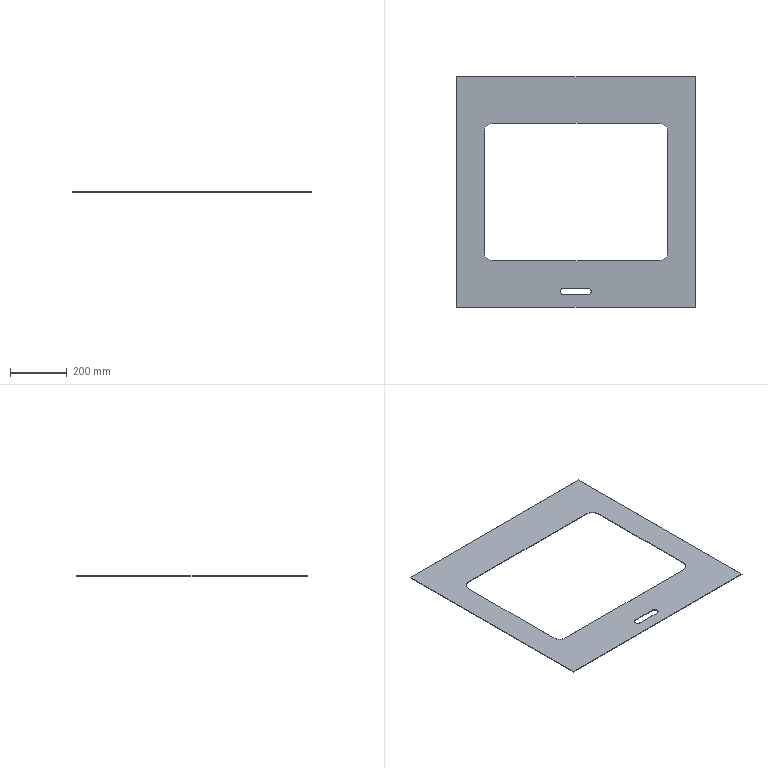Part | STEP file | Plate金1-2^B9CHAO000_ASM-2 | 1 solid | 19 faces | box 846 x 816 x 2 mm | volume 745734 mm3 | plane 12 | cylinder 7 | commonest cylinder face diameters 60 x4 24.334 x3
STEP:
#1=CARTESIAN_POINT('',(-370.911,77.769,-2.));
#2=VERTEX_POINT('',#1);
#3=CARTESIAN_POINT('',(-383.079,89.936,-2.));
#4=VERTEX_POINT('',#3);
#5=CARTESIAN_POINT('',(-383.079,77.769,-2.));
#6=DIRECTION('',(0.,0.,1.));
#7=DIRECTION('',(1.,0.,0.));
#8=AXIS2_PLACEMENT_3D('',#5,#6,#7);
#9=CIRCLE('',#8,12.167);
#10=EDGE_CURVE('',#2,#4,#9,.T.);
#11=ORIENTED_EDGE('',*,*,#10,.F.);
#12=CARTESIAN_POINT('',(-370.911,77.769,0.));
#13=VERTEX_POINT('',#12);
#14=CARTESIAN_POINT('',(-370.911,77.769,-2.));
#15=DIRECTION('',(0.,0.,1.));
#16=VECTOR('',#15,1000.);
#17=LINE('',#14,#16);
#18=EDGE_CURVE('',#2,#13,#17,.T.);
#19=ORIENTED_EDGE('',*,*,#18,.T.);
#20=CARTESIAN_POINT('',(-383.079,89.936,0.));
#21=VERTEX_POINT('',#20);
#22=CARTESIAN_POINT('',(-383.079,77.769,0.));
#23=DIRECTION('',(0.,0.,1.));
#24=DIRECTION('',(1.,0.,0.));
#25=AXIS2_PLACEMENT_3D('',#22,#23,#24);
#26=CIRCLE('',#25,12.167);
#27=EDGE_CURVE('',#13,#21,#26,.T.);
#28=ORIENTED_EDGE('',*,*,#27,.T.);
#29=CARTESIAN_POINT('',(-383.079,89.936,-2.));
#30=DIRECTION('',(0.,0.,1.));
#31=VECTOR('',#30,1000.);
#32=LINE('',#29,#31);
#33=EDGE_CURVE('',#4,#21,#32,.T.);
#34=ORIENTED_EDGE('',*,*,#33,.F.);
#35=EDGE_LOOP('',(#11,#19,#28,#34));
#36=FACE_OUTER_BOUND('',#35,.T.);
#37=CARTESIAN_POINT('',(-383.079,77.769,-2.));
#38=DIRECTION('',(0.,0.,1.));
#39=DIRECTION('',(1.,0.,0.));
#40=AXIS2_PLACEMENT_3D('',#37,#38,#39);
#41=CYLINDRICAL_SURFACE('',#40,12.167);
#42=ADVANCED_FACE('',(#36),#41,.F.);
#43=CARTESIAN_POINT('',(-2.,838.,0.));
#44=VERTEX_POINT('',#43);
#45=CARTESIAN_POINT('',(-848.,838.,0.));
#46=VERTEX_POINT('',#45);
#47=CARTESIAN_POINT('',(-848.,838.,0.));
#48=DIRECTION('',(-1.,0.,0.));
#49=VECTOR('',#48,1000.);
#50=LINE('',#47,#49);
#51=EDGE_CURVE('',#44,#46,#50,.T.);
#52=ORIENTED_EDGE('',*,*,#51,.F.);
#53=CARTESIAN_POINT('',(-2.,838.,-2.));
#54=VERTEX_POINT('',#53);
#55=CARTESIAN_POINT('',(-2.,838.,-2.));
#56=DIRECTION('',(0.,0.,1.));
#57=VECTOR('',#56,1000.);
#58=LINE('',#55,#57);
#59=EDGE_CURVE('',#54,#44,#58,.T.);
#60=ORIENTED_EDGE('',*,*,#59,.F.);
#61=CARTESIAN_POINT('',(-848.,838.,-2.));
#62=VERTEX_POINT('',#61);
#63=CARTESIAN_POINT('',(-848.,838.,-2.));
#64=DIRECTION('',(-1.,0.,0.));
#65=VECTOR('',#64,1000.);
#66=LINE('',#63,#65);
#67=EDGE_CURVE('',#54,#62,#66,.T.);
#68=ORIENTED_EDGE('',*,*,#67,.T.);
#69=CARTESIAN_POINT('',(-848.,838.,-2.));
#70=DIRECTION('',(0.,0.,1.));
#71=VECTOR('',#70,1000.);
#72=LINE('',#69,#71);
#73=EDGE_CURVE('',#62,#46,#72,.T.);
#74=ORIENTED_EDGE('',*,*,#73,.T.);
#75=EDGE_LOOP('',(#52,#60,#68,#74));
#76=FACE_OUTER_BOUND('',#75,.T.);
#77=CARTESIAN_POINT('',(-848.,838.,-2.));
#78=DIRECTION('',(0.,1.,0.));
#79=DIRECTION('',(0.,0.,1.));
#80=AXIS2_PLACEMENT_3D('',#77,#78,#79);
#81=PLANE('',#80);
#82=ADVANCED_FACE('',(#76),#81,.T.);
#83=CARTESIAN_POINT('',(-2.,22.,0.));
#84=VERTEX_POINT('',#83);
#85=CARTESIAN_POINT('',(-2.,838.,0.));
#86=DIRECTION('',(0.,1.,0.));
#87=VECTOR('',#86,1000.);
#88=LINE('',#85,#87);
#89=EDGE_CURVE('',#84,#44,#88,.T.);
#90=ORIENTED_EDGE('',*,*,#89,.F.);
#91=CARTESIAN_POINT('',(-2.,22.,-2.));
#92=VERTEX_POINT('',#91);
#93=CARTESIAN_POINT('',(-2.,22.,-2.));
#94=DIRECTION('',(0.,0.,1.));
#95=VECTOR('',#94,1000.);
#96=LINE('',#93,#95);
#97=EDGE_CURVE('',#92,#84,#96,.T.);
#98=ORIENTED_EDGE('',*,*,#97,.F.);
#99=CARTESIAN_POINT('',(-2.,838.,-2.));
#100=DIRECTION('',(0.,1.,0.));
#101=VECTOR('',#100,1000.);
#102=LINE('',#99,#101);
#103=EDGE_CURVE('',#92,#54,#102,.T.);
#104=ORIENTED_EDGE('',*,*,#103,.T.);
#105=ORIENTED_EDGE('',*,*,#59,.T.);
#106=EDGE_LOOP('',(#90,#98,#104,#105));
#107=FACE_OUTER_BOUND('',#106,.T.);
#108=CARTESIAN_POINT('',(-2.,838.,-2.));
#109=DIRECTION('',(1.,0.,0.));
#110=DIRECTION('',(0.,1.,0.));
#111=AXIS2_PLACEMENT_3D('',#108,#109,#110);
#112=PLANE('',#111);
#113=ADVANCED_FACE('',(#107),#112,.T.);
#114=CARTESIAN_POINT('',(-848.,22.,0.));
#115=VERTEX_POINT('',#114);
#116=CARTESIAN_POINT('',(-848.,22.,0.));
#117=DIRECTION('',(1.,0.,0.));
#118=VECTOR('',#117,1000.);
#119=LINE('',#116,#118);
#120=EDGE_CURVE('',#115,#84,#119,.T.);
#121=ORIENTED_EDGE('',*,*,#120,.F.);
#122=CARTESIAN_POINT('',(-848.,22.,-2.));
#123=VERTEX_POINT('',#122);
#124=CARTESIAN_POINT('',(-848.,22.,-2.));
#125=DIRECTION('',(0.,0.,1.));
#126=VECTOR('',#125,1000.);
#127=LINE('',#124,#126);
#128=EDGE_CURVE('',#123,#115,#127,.T.);
#129=ORIENTED_EDGE('',*,*,#128,.F.);
#130=CARTESIAN_POINT('',(-848.,22.,-2.));
#131=DIRECTION('',(1.,0.,0.));
#132=VECTOR('',#131,1000.);
#133=LINE('',#130,#132);
#134=EDGE_CURVE('',#123,#92,#133,.T.);
#135=ORIENTED_EDGE('',*,*,#134,.T.);
#136=ORIENTED_EDGE('',*,*,#97,.T.);
#137=EDGE_LOOP('',(#121,#129,#135,#136));
#138=FACE_OUTER_BOUND('',#137,.T.);
#139=CARTESIAN_POINT('',(-848.,22.,-2.));
#140=DIRECTION('',(0.,-1.,0.));
#141=DIRECTION('',(0.,0.,-1.));
#142=AXIS2_PLACEMENT_3D('',#139,#140,#141);
#143=PLANE('',#142);
#144=ADVANCED_FACE('',(#138),#143,.T.);
#145=CARTESIAN_POINT('',(-848.,838.,0.));
#146=DIRECTION('',(0.,-1.,0.));
#147=VECTOR('',#146,1000.);
#148=LINE('',#145,#147);
#149=EDGE_CURVE('',#46,#115,#148,.T.);
#150=ORIENTED_EDGE('',*,*,#149,.F.);
#151=ORIENTED_EDGE('',*,*,#73,.F.);
#152=CARTESIAN_POINT('',(-848.,838.,-2.));
#153=DIRECTION('',(0.,-1.,0.));
#154=VECTOR('',#153,1000.);
#155=LINE('',#152,#154);
#156=EDGE_CURVE('',#62,#123,#155,.T.);
#157=ORIENTED_EDGE('',*,*,#156,.T.);
#158=ORIENTED_EDGE('',*,*,#128,.T.);
#159=EDGE_LOOP('',(#150,#151,#157,#158));
#160=FACE_OUTER_BOUND('',#159,.T.);
#161=CARTESIAN_POINT('',(-848.,838.,-2.));
#162=DIRECTION('',(-1.,0.,0.));
#163=DIRECTION('',(0.,0.,1.));
#164=AXIS2_PLACEMENT_3D('',#161,#162,#163);
#165=PLANE('',#164);
#166=ADVANCED_FACE('',(#160),#165,.T.);
#167=CARTESIAN_POINT('',(-383.079,65.602,-2.));
#168=VERTEX_POINT('',#167);
#169=CARTESIAN_POINT('',(-383.079,77.769,-2.));
#170=DIRECTION('',(0.,0.,1.));
#171=DIRECTION('',(1.,0.,0.));
#172=AXIS2_PLACEMENT_3D('',#169,#170,#171);
#173=CIRCLE('',#172,12.167);
#174=EDGE_CURVE('',#168,#2,#173,.T.);
#175=ORIENTED_EDGE('',*,*,#174,.T.);
#176=ORIENTED_EDGE('',*,*,#10,.T.);
#177=CARTESIAN_POINT('',(-466.921,89.936,-2.));
#178=VERTEX_POINT('',#177);
#179=CARTESIAN_POINT('',(-383.079,89.936,-2.));
#180=DIRECTION('',(-1.,0.,0.));
#181=VECTOR('',#180,1000.);
#182=LINE('',#179,#181);
#183=EDGE_CURVE('',#4,#178,#182,.T.);
#184=ORIENTED_EDGE('',*,*,#183,.T.);
#185=CARTESIAN_POINT('',(-466.921,65.602,-2.));
#186=VERTEX_POINT('',#185);
#187=CARTESIAN_POINT('',(-466.921,77.769,-2.));
#188=DIRECTION('',(0.,0.,1.));
#189=DIRECTION('',(1.,0.,0.));
#190=AXIS2_PLACEMENT_3D('',#187,#188,#189);
#191=CIRCLE('',#190,12.167);
#192=EDGE_CURVE('',#178,#186,#191,.T.);
#193=ORIENTED_EDGE('',*,*,#192,.T.);
#194=CARTESIAN_POINT('',(-383.079,65.602,-2.));
#195=DIRECTION('',(1.,0.,0.));
#196=VECTOR('',#195,1000.);
#197=LINE('',#194,#196);
#198=EDGE_CURVE('',#186,#168,#197,.T.);
#199=ORIENTED_EDGE('',*,*,#198,.T.);
#200=EDGE_LOOP('',(#175,#176,#184,#193,#199));
#201=FACE_BOUND('',#200,.T.);
#202=CARTESIAN_POINT('',(-750.213,217.285,-2.));
#203=VERTEX_POINT('',#202);
#204=CARTESIAN_POINT('',(-720.213,187.285,-2.));
#205=VERTEX_POINT('',#204);
#206=CARTESIAN_POINT('',(-720.213,217.285,-2.));
#207=DIRECTION('',(0.,0.,1.));
#208=DIRECTION('',(1.,0.,0.));
#209=AXIS2_PLACEMENT_3D('',#206,#207,#208);
#210=CIRCLE('',#209,30.);
#211=EDGE_CURVE('',#203,#205,#210,.T.);
#212=ORIENTED_EDGE('',*,*,#211,.T.);
#213=CARTESIAN_POINT('',(-129.787,187.285,-2.));
#214=VERTEX_POINT('',#213);
#215=CARTESIAN_POINT('',(-720.213,187.285,-2.));
#216=DIRECTION('',(1.,0.,0.));
#217=VECTOR('',#216,1000.);
#218=LINE('',#215,#217);
#219=EDGE_CURVE('',#205,#214,#218,.T.);
#220=ORIENTED_EDGE('',*,*,#219,.T.);
#221=CARTESIAN_POINT('',(-99.787,217.285,-2.));
#222=VERTEX_POINT('',#221);
#223=CARTESIAN_POINT('',(-129.787,217.285,-2.));
#224=DIRECTION('',(0.,0.,1.));
#225=DIRECTION('',(1.,0.,0.));
#226=AXIS2_PLACEMENT_3D('',#223,#224,#225);
#227=CIRCLE('',#226,30.);
#228=EDGE_CURVE('',#214,#222,#227,.T.);
#229=ORIENTED_EDGE('',*,*,#228,.T.);
#230=CARTESIAN_POINT('',(-99.787,642.715,-2.));
#231=VERTEX_POINT('',#230);
#232=CARTESIAN_POINT('',(-99.787,217.285,-2.));
#233=DIRECTION('',(0.,1.,0.));
#234=VECTOR('',#233,1000.);
#235=LINE('',#232,#234);
#236=EDGE_CURVE('',#222,#231,#235,.T.);
#237=ORIENTED_EDGE('',*,*,#236,.T.);
#238=CARTESIAN_POINT('',(-129.787,672.715,-2.));
#239=VERTEX_POINT('',#238);
#240=CARTESIAN_POINT('',(-129.787,642.715,-2.));
#241=DIRECTION('',(0.,0.,1.));
#242=DIRECTION('',(1.,0.,0.));
#243=AXIS2_PLACEMENT_3D('',#240,#241,#242);
#244=CIRCLE('',#243,30.);
#245=EDGE_CURVE('',#231,#239,#244,.T.);
#246=ORIENTED_EDGE('',*,*,#245,.T.);
#247=CARTESIAN_POINT('',(-720.213,672.715,-2.));
#248=VERTEX_POINT('',#247);
#249=CARTESIAN_POINT('',(-720.213,672.715,-2.));
#250=DIRECTION('',(-1.,0.,0.));
#251=VECTOR('',#250,1000.);
#252=LINE('',#249,#251);
#253=EDGE_CURVE('',#239,#248,#252,.T.);
#254=ORIENTED_EDGE('',*,*,#253,.T.);
#255=CARTESIAN_POINT('',(-750.213,642.715,-2.));
#256=VERTEX_POINT('',#255);
#257=CARTESIAN_POINT('',(-720.213,642.715,-2.));
#258=DIRECTION('',(0.,0.,1.));
#259=DIRECTION('',(-1.,0.,0.));
#260=AXIS2_PLACEMENT_3D('',#257,#258,#259);
#261=CIRCLE('',#260,30.);
#262=EDGE_CURVE('',#248,#256,#261,.T.);
#263=ORIENTED_EDGE('',*,*,#262,.T.);
#264=CARTESIAN_POINT('',(-750.213,217.285,-2.));
#265=DIRECTION('',(0.,-1.,0.));
#266=VECTOR('',#265,1000.);
#267=LINE('',#264,#266);
#268=EDGE_CURVE('',#256,#203,#267,.T.);
#269=ORIENTED_EDGE('',*,*,#268,.T.);
#270=EDGE_LOOP('',(#212,#220,#229,#237,#246,#254,#263,#269));
#271=FACE_BOUND('',#270,.T.);
#272=ORIENTED_EDGE('',*,*,#67,.F.);
#273=ORIENTED_EDGE('',*,*,#103,.F.);
#274=ORIENTED_EDGE('',*,*,#134,.F.);
#275=ORIENTED_EDGE('',*,*,#156,.F.);
#276=EDGE_LOOP('',(#272,#273,#274,#275));
#277=FACE_OUTER_BOUND('',#276,.T.);
#278=CARTESIAN_POINT('',(-2.,838.,-2.));
#279=DIRECTION('',(0.,0.,-1.));
#280=DIRECTION('',(-1.,0.,0.));
#281=AXIS2_PLACEMENT_3D('',#278,#279,#280);
#282=PLANE('',#281);
#283=ADVANCED_FACE('',(#201,#271,#277),#282,.T.);
#284=CARTESIAN_POINT('',(-466.921,89.936,0.));
#285=VERTEX_POINT('',#284);
#286=CARTESIAN_POINT('',(-383.079,89.936,0.));
#287=DIRECTION('',(-1.,0.,0.));
#288=VECTOR('',#287,1000.);
#289=LINE('',#286,#288);
#290=EDGE_CURVE('',#21,#285,#289,.T.);
#291=ORIENTED_EDGE('',*,*,#290,.F.);
#292=ORIENTED_EDGE('',*,*,#27,.F.);
#293=CARTESIAN_POINT('',(-383.079,65.602,0.));
#294=VERTEX_POINT('',#293);
#295=CARTESIAN_POINT('',(-383.079,77.769,0.));
#296=DIRECTION('',(0.,0.,1.));
#297=DIRECTION('',(1.,0.,0.));
#298=AXIS2_PLACEMENT_3D('',#295,#296,#297);
#299=CIRCLE('',#298,12.167);
#300=EDGE_CURVE('',#294,#13,#299,.T.);
#301=ORIENTED_EDGE('',*,*,#300,.F.);
#302=CARTESIAN_POINT('',(-466.921,65.602,0.));
#303=VERTEX_POINT('',#302);
#304=CARTESIAN_POINT('',(-383.079,65.602,0.));
#305=DIRECTION('',(1.,0.,0.));
#306=VECTOR('',#305,1000.);
#307=LINE('',#304,#306);
#308=EDGE_CURVE('',#303,#294,#307,.T.);
#309=ORIENTED_EDGE('',*,*,#308,.F.);
#310=CARTESIAN_POINT('',(-466.921,77.769,0.));
#311=DIRECTION('',(0.,0.,1.));
#312=DIRECTION('',(1.,0.,0.));
#313=AXIS2_PLACEMENT_3D('',#310,#311,#312);
#314=CIRCLE('',#313,12.167);
#315=EDGE_CURVE('',#285,#303,#314,.T.);
#316=ORIENTED_EDGE('',*,*,#315,.F.);
#317=EDGE_LOOP('',(#291,#292,#301,#309,#316));
#318=FACE_BOUND('',#317,.T.);
#319=CARTESIAN_POINT('',(-720.213,187.285,0.));
#320=VERTEX_POINT('',#319);
#321=CARTESIAN_POINT('',(-129.787,187.285,0.));
#322=VERTEX_POINT('',#321);
#323=CARTESIAN_POINT('',(-720.213,187.285,0.));
#324=DIRECTION('',(1.,0.,0.));
#325=VECTOR('',#324,1000.);
#326=LINE('',#323,#325);
#327=EDGE_CURVE('',#320,#322,#326,.T.);
#328=ORIENTED_EDGE('',*,*,#327,.F.);
#329=CARTESIAN_POINT('',(-750.213,217.285,0.));
#330=VERTEX_POINT('',#329);
#331=CARTESIAN_POINT('',(-720.213,217.285,0.));
#332=DIRECTION('',(0.,0.,1.));
#333=DIRECTION('',(1.,0.,0.));
#334=AXIS2_PLACEMENT_3D('',#331,#332,#333);
#335=CIRCLE('',#334,30.);
#336=EDGE_CURVE('',#330,#320,#335,.T.);
#337=ORIENTED_EDGE('',*,*,#336,.F.);
#338=CARTESIAN_POINT('',(-750.213,642.715,0.));
#339=VERTEX_POINT('',#338);
#340=CARTESIAN_POINT('',(-750.213,217.285,0.));
#341=DIRECTION('',(0.,-1.,0.));
#342=VECTOR('',#341,1000.);
#343=LINE('',#340,#342);
#344=EDGE_CURVE('',#339,#330,#343,.T.);
#345=ORIENTED_EDGE('',*,*,#344,.F.);
#346=CARTESIAN_POINT('',(-720.213,672.715,0.));
#347=VERTEX_POINT('',#346);
#348=CARTESIAN_POINT('',(-720.213,642.715,0.));
#349=DIRECTION('',(0.,0.,1.));
#350=DIRECTION('',(-1.,0.,0.));
#351=AXIS2_PLACEMENT_3D('',#348,#349,#350);
#352=CIRCLE('',#351,30.);
#353=EDGE_CURVE('',#347,#339,#352,.T.);
#354=ORIENTED_EDGE('',*,*,#353,.F.);
#355=CARTESIAN_POINT('',(-129.787,672.715,0.));
#356=VERTEX_POINT('',#355);
#357=CARTESIAN_POINT('',(-720.213,672.715,0.));
#358=DIRECTION('',(-1.,0.,0.));
#359=VECTOR('',#358,1000.);
#360=LINE('',#357,#359);
#361=EDGE_CURVE('',#356,#347,#360,.T.);
#362=ORIENTED_EDGE('',*,*,#361,.F.);
#363=CARTESIAN_POINT('',(-99.787,642.715,0.));
#364=VERTEX_POINT('',#363);
#365=CARTESIAN_POINT('',(-129.787,642.715,0.));
#366=DIRECTION('',(0.,0.,1.));
#367=DIRECTION('',(1.,0.,0.));
#368=AXIS2_PLACEMENT_3D('',#365,#366,#367);
#369=CIRCLE('',#368,30.);
#370=EDGE_CURVE('',#364,#356,#369,.T.);
#371=ORIENTED_EDGE('',*,*,#370,.F.);
#372=CARTESIAN_POINT('',(-99.787,217.285,0.));
#373=VERTEX_POINT('',#372);
#374=CARTESIAN_POINT('',(-99.787,217.285,0.));
#375=DIRECTION('',(0.,1.,0.));
#376=VECTOR('',#375,1000.);
#377=LINE('',#374,#376);
#378=EDGE_CURVE('',#373,#364,#377,.T.);
#379=ORIENTED_EDGE('',*,*,#378,.F.);
#380=CARTESIAN_POINT('',(-129.787,217.285,0.));
#381=DIRECTION('',(0.,0.,1.));
#382=DIRECTION('',(1.,0.,0.));
#383=AXIS2_PLACEMENT_3D('',#380,#381,#382);
#384=CIRCLE('',#383,30.);
#385=EDGE_CURVE('',#322,#373,#384,.T.);
#386=ORIENTED_EDGE('',*,*,#385,.F.);
#387=EDGE_LOOP('',(#328,#337,#345,#354,#362,#371,#379,#386));
#388=FACE_BOUND('',#387,.T.);
#389=ORIENTED_EDGE('',*,*,#51,.T.);
#390=ORIENTED_EDGE('',*,*,#149,.T.);
#391=ORIENTED_EDGE('',*,*,#120,.T.);
#392=ORIENTED_EDGE('',*,*,#89,.T.);
#393=EDGE_LOOP('',(#389,#390,#391,#392));
#394=FACE_OUTER_BOUND('',#393,.T.);
#395=CARTESIAN_POINT('',(-2.,838.,0.));
#396=DIRECTION('',(0.,0.,-1.));
#397=DIRECTION('',(-1.,0.,0.));
#398=AXIS2_PLACEMENT_3D('',#395,#396,#397);
#399=PLANE('',#398);
#400=ADVANCED_FACE('',(#318,#388,#394),#399,.F.);
#401=ORIENTED_EDGE('',*,*,#336,.T.);
#402=CARTESIAN_POINT('',(-720.213,187.285,-2.));
#403=DIRECTION('',(0.,0.,1.));
#404=VECTOR('',#403,1000.);
#405=LINE('',#402,#404);
#406=EDGE_CURVE('',#205,#320,#405,.T.);
#407=ORIENTED_EDGE('',*,*,#406,.F.);
#408=ORIENTED_EDGE('',*,*,#211,.F.);
#409=CARTESIAN_POINT('',(-750.213,217.285,-2.));
#410=DIRECTION('',(0.,0.,1.));
#411=VECTOR('',#410,1000.);
#412=LINE('',#409,#411);
#413=EDGE_CURVE('',#203,#330,#412,.T.);
#414=ORIENTED_EDGE('',*,*,#413,.T.);
#415=EDGE_LOOP('',(#401,#407,#408,#414));
#416=FACE_OUTER_BOUND('',#415,.T.);
#417=CARTESIAN_POINT('',(-720.213,217.285,-2.));
#418=DIRECTION('',(0.,0.,1.));
#419=DIRECTION('',(1.,0.,0.));
#420=AXIS2_PLACEMENT_3D('',#417,#418,#419);
#421=CYLINDRICAL_SURFACE('',#420,30.);
#422=ADVANCED_FACE('',(#416),#421,.F.);
#423=ORIENTED_EDGE('',*,*,#344,.T.);
#424=ORIENTED_EDGE('',*,*,#413,.F.);
#425=ORIENTED_EDGE('',*,*,#268,.F.);
#426=CARTESIAN_POINT('',(-750.213,642.715,-2.));
#427=DIRECTION('',(0.,0.,1.));
#428=VECTOR('',#427,1000.);
#429=LINE('',#426,#428);
#430=EDGE_CURVE('',#256,#339,#429,.T.);
#431=ORIENTED_EDGE('',*,*,#430,.T.);
#432=EDGE_LOOP('',(#423,#424,#425,#431));
#433=FACE_OUTER_BOUND('',#432,.T.);
#434=CARTESIAN_POINT('',(-750.213,217.285,-2.));
#435=DIRECTION('',(-1.,0.,0.));
#436=DIRECTION('',(0.,0.,1.));
#437=AXIS2_PLACEMENT_3D('',#434,#435,#436);
#438=PLANE('',#437);
#439=ADVANCED_FACE('',(#433),#438,.F.);
#440=ORIENTED_EDGE('',*,*,#353,.T.);
#441=ORIENTED_EDGE('',*,*,#430,.F.);
#442=ORIENTED_EDGE('',*,*,#262,.F.);
#443=CARTESIAN_POINT('',(-720.213,672.715,-2.));
#444=DIRECTION('',(0.,0.,1.));
#445=VECTOR('',#444,1000.);
#446=LINE('',#443,#445);
#447=EDGE_CURVE('',#248,#347,#446,.T.);
#448=ORIENTED_EDGE('',*,*,#447,.T.);
#449=EDGE_LOOP('',(#440,#441,#442,#448));
#450=FACE_OUTER_BOUND('',#449,.T.);
#451=CARTESIAN_POINT('',(-720.213,642.715,-2.));
#452=DIRECTION('',(0.,0.,1.));
#453=DIRECTION('',(1.,0.,0.));
#454=AXIS2_PLACEMENT_3D('',#451,#452,#453);
#455=CYLINDRICAL_SURFACE('',#454,30.);
#456=ADVANCED_FACE('',(#450),#455,.F.);
#457=ORIENTED_EDGE('',*,*,#361,.T.);
#458=ORIENTED_EDGE('',*,*,#447,.F.);
#459=ORIENTED_EDGE('',*,*,#253,.F.);
#460=CARTESIAN_POINT('',(-129.787,672.715,-2.));
#461=DIRECTION('',(0.,0.,1.));
#462=VECTOR('',#461,1000.);
#463=LINE('',#460,#462);
#464=EDGE_CURVE('',#239,#356,#463,.T.);
#465=ORIENTED_EDGE('',*,*,#464,.T.);
#466=EDGE_LOOP('',(#457,#458,#459,#465));
#467=FACE_OUTER_BOUND('',#466,.T.);
#468=CARTESIAN_POINT('',(-720.213,672.715,-2.));
#469=DIRECTION('',(0.,1.,0.));
#470=DIRECTION('',(0.,0.,1.));
#471=AXIS2_PLACEMENT_3D('',#468,#469,#470);
#472=PLANE('',#471);
#473=ADVANCED_FACE('',(#467),#472,.F.);
#474=ORIENTED_EDGE('',*,*,#370,.T.);
#475=ORIENTED_EDGE('',*,*,#464,.F.);
#476=ORIENTED_EDGE('',*,*,#245,.F.);
#477=CARTESIAN_POINT('',(-99.787,642.715,-2.));
#478=DIRECTION('',(0.,0.,1.));
#479=VECTOR('',#478,1000.);
#480=LINE('',#477,#479);
#481=EDGE_CURVE('',#231,#364,#480,.T.);
#482=ORIENTED_EDGE('',*,*,#481,.T.);
#483=EDGE_LOOP('',(#474,#475,#476,#482));
#484=FACE_OUTER_BOUND('',#483,.T.);
#485=CARTESIAN_POINT('',(-129.787,642.715,-2.));
#486=DIRECTION('',(0.,0.,1.));
#487=DIRECTION('',(1.,0.,0.));
#488=AXIS2_PLACEMENT_3D('',#485,#486,#487);
#489=CYLINDRICAL_SURFACE('',#488,30.);
#490=ADVANCED_FACE('',(#484),#489,.F.);
#491=ORIENTED_EDGE('',*,*,#378,.T.);
#492=ORIENTED_EDGE('',*,*,#481,.F.);
#493=ORIENTED_EDGE('',*,*,#236,.F.);
#494=CARTESIAN_POINT('',(-99.787,217.285,-2.));
#495=DIRECTION('',(0.,0.,1.));
#496=VECTOR('',#495,1000.);
#497=LINE('',#494,#496);
#498=EDGE_CURVE('',#222,#373,#497,.T.);
#499=ORIENTED_EDGE('',*,*,#498,.T.);
#500=EDGE_LOOP('',(#491,#492,#493,#499));
#501=FACE_OUTER_BOUND('',#500,.T.);
#502=CARTESIAN_POINT('',(-99.787,217.285,-2.));
#503=DIRECTION('',(1.,0.,0.));
#504=DIRECTION('',(0.,0.,-1.));
#505=AXIS2_PLACEMENT_3D('',#502,#503,#504);
#506=PLANE('',#505);
#507=ADVANCED_FACE('',(#501),#506,.F.);
#508=ORIENTED_EDGE('',*,*,#385,.T.);
#509=ORIENTED_EDGE('',*,*,#498,.F.);
#510=ORIENTED_EDGE('',*,*,#228,.F.);
#511=CARTESIAN_POINT('',(-129.787,187.285,-2.));
#512=DIRECTION('',(0.,0.,1.));
#513=VECTOR('',#512,1000.);
#514=LINE('',#511,#513);
#515=EDGE_CURVE('',#214,#322,#514,.T.);
#516=ORIENTED_EDGE('',*,*,#515,.T.);
#517=EDGE_LOOP('',(#508,#509,#510,#516));
#518=FACE_OUTER_BOUND('',#517,.T.);
#519=CARTESIAN_POINT('',(-129.787,217.285,-2.));
#520=DIRECTION('',(0.,0.,1.));
#521=DIRECTION('',(1.,0.,0.));
#522=AXIS2_PLACEMENT_3D('',#519,#520,#521);
#523=CYLINDRICAL_SURFACE('',#522,30.);
#524=ADVANCED_FACE('',(#518),#523,.F.);
#525=ORIENTED_EDGE('',*,*,#327,.T.);
#526=ORIENTED_EDGE('',*,*,#515,.F.);
#527=ORIENTED_EDGE('',*,*,#219,.F.);
#528=ORIENTED_EDGE('',*,*,#406,.T.);
#529=EDGE_LOOP('',(#525,#526,#527,#528));
#530=FACE_OUTER_BOUND('',#529,.T.);
#531=CARTESIAN_POINT('',(-720.213,187.285,-2.));
#532=DIRECTION('',(0.,-1.,0.));
#533=DIRECTION('',(0.,0.,-1.));
#534=AXIS2_PLACEMENT_3D('',#531,#532,#533);
#535=PLANE('',#534);
#536=ADVANCED_FACE('',(#530),#535,.F.);
#537=ORIENTED_EDGE('',*,*,#18,.F.);
#538=ORIENTED_EDGE('',*,*,#174,.F.);
#539=CARTESIAN_POINT('',(-383.079,65.602,-2.));
#540=DIRECTION('',(0.,0.,1.));
#541=VECTOR('',#540,1000.);
#542=LINE('',#539,#541);
#543=EDGE_CURVE('',#168,#294,#542,.T.);
#544=ORIENTED_EDGE('',*,*,#543,.T.);
#545=ORIENTED_EDGE('',*,*,#300,.T.);
#546=EDGE_LOOP('',(#537,#538,#544,#545));
#547=FACE_OUTER_BOUND('',#546,.T.);
#548=CARTESIAN_POINT('',(-383.079,77.769,-2.));
#549=DIRECTION('',(0.,0.,1.));
#550=DIRECTION('',(1.,0.,0.));
#551=AXIS2_PLACEMENT_3D('',#548,#549,#550);
#552=CYLINDRICAL_SURFACE('',#551,12.167);
#553=ADVANCED_FACE('',(#547),#552,.F.);
#554=ORIENTED_EDGE('',*,*,#308,.T.);
#555=ORIENTED_EDGE('',*,*,#543,.F.);
#556=ORIENTED_EDGE('',*,*,#198,.F.);
#557=CARTESIAN_POINT('',(-466.921,65.602,-2.));
#558=DIRECTION('',(0.,0.,1.));
#559=VECTOR('',#558,1000.);
#560=LINE('',#557,#559);
#561=EDGE_CURVE('',#186,#303,#560,.T.);
#562=ORIENTED_EDGE('',*,*,#561,.T.);
#563=EDGE_LOOP('',(#554,#555,#556,#562));
#564=FACE_OUTER_BOUND('',#563,.T.);
#565=CARTESIAN_POINT('',(-383.079,65.602,-2.));
#566=DIRECTION('',(0.,-1.,0.));
#567=DIRECTION('',(0.,0.,-1.));
#568=AXIS2_PLACEMENT_3D('',#565,#566,#567);
#569=PLANE('',#568);
#570=ADVANCED_FACE('',(#564),#569,.F.);
#571=ORIENTED_EDGE('',*,*,#315,.T.);
#572=ORIENTED_EDGE('',*,*,#561,.F.);
#573=ORIENTED_EDGE('',*,*,#192,.F.);
#574=CARTESIAN_POINT('',(-466.921,89.936,-2.));
#575=DIRECTION('',(0.,0.,1.));
#576=VECTOR('',#575,1000.);
#577=LINE('',#574,#576);
#578=EDGE_CURVE('',#178,#285,#577,.T.);
#579=ORIENTED_EDGE('',*,*,#578,.T.);
#580=EDGE_LOOP('',(#571,#572,#573,#579));
#581=FACE_OUTER_BOUND('',#580,.T.);
#582=CARTESIAN_POINT('',(-466.921,77.769,-2.));
#583=DIRECTION('',(0.,0.,1.));
#584=DIRECTION('',(1.,0.,0.));
#585=AXIS2_PLACEMENT_3D('',#582,#583,#584);
#586=CYLINDRICAL_SURFACE('',#585,12.167);
#587=ADVANCED_FACE('',(#581),#586,.F.);
#588=ORIENTED_EDGE('',*,*,#290,.T.);
#589=ORIENTED_EDGE('',*,*,#578,.F.);
#590=ORIENTED_EDGE('',*,*,#183,.F.);
#591=ORIENTED_EDGE('',*,*,#33,.T.);
#592=EDGE_LOOP('',(#588,#589,#590,#591));
#593=FACE_OUTER_BOUND('',#592,.T.);
#594=CARTESIAN_POINT('',(-383.079,89.936,-2.));
#595=DIRECTION('',(0.,1.,0.));
#596=DIRECTION('',(0.,0.,1.));
#597=AXIS2_PLACEMENT_3D('',#594,#595,#596);
#598=PLANE('',#597);
#599=ADVANCED_FACE('',(#593),#598,.F.);
#600=CLOSED_SHELL('',(#42,#82,#113,#144,#166,#283,#400,#422,#439,#456,#473,#490,#507,#524,#536,#553,#570,#587,#599));
#601=MANIFOLD_SOLID_BREP('',#600);
#602=CARTESIAN_POINT('',(0.,0.,0.));
#603=DIRECTION('',(0.,0.,1.));
#604=DIRECTION('',(1.,0.,0.));
#605=AXIS2_PLACEMENT_3D('',#602,#603,#604);
#606=(LENGTH_UNIT()NAMED_UNIT(*)SI_UNIT(.MILLI.,.METRE.));
#607=UNCERTAINTY_MEASURE_WITH_UNIT(LENGTH_MEASURE(0.00001),#606,'','');
#608=(NAMED_UNIT(*)PLANE_ANGLE_UNIT()SI_UNIT($,.RADIAN.));
#609=(NAMED_UNIT(*)SI_UNIT($,.STERADIAN.)SOLID_ANGLE_UNIT());
#610=(GEOMETRIC_REPRESENTATION_CONTEXT(3)GLOBAL_UNCERTAINTY_ASSIGNED_CONTEXT((#607))GLOBAL_UNIT_ASSIGNED_CONTEXT((#606,#608,#609))REPRESENTATION_CONTEXT('',''));
#611=ADVANCED_BREP_SHAPE_REPRESENTATION('',(#601,#605),#610);